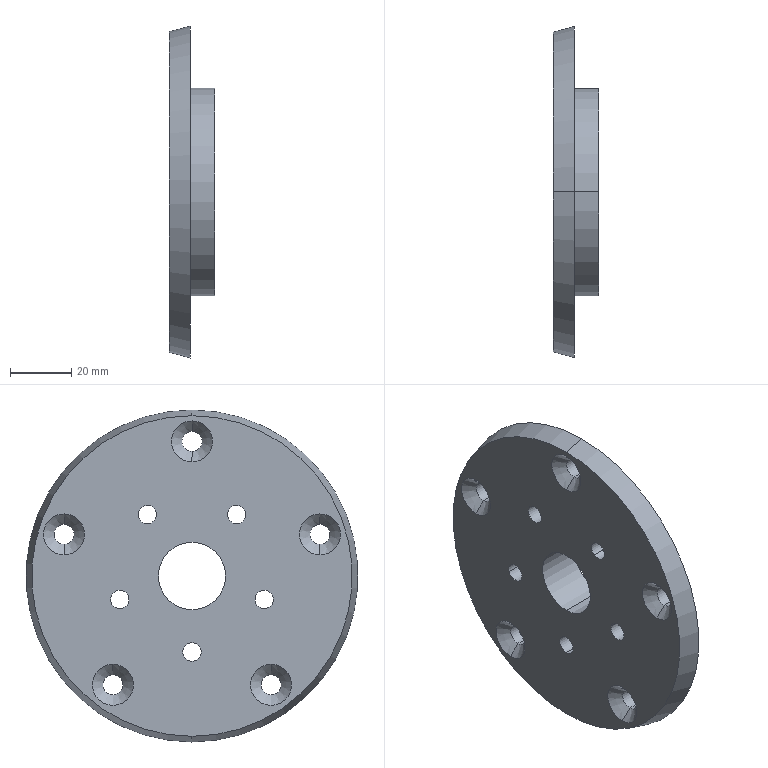Part | STEP file | Previa 01.sldasm-Part-6_Valor predeterminado | 1 solid | 39 faces | box 15 x 108.559 x 108.559 mm | volume 81796 mm3 | cylinder 24 | cone 12 | plane 3 | commonest cylinder face diameters 6 x10 6.6 x10 22 x2 68 x2